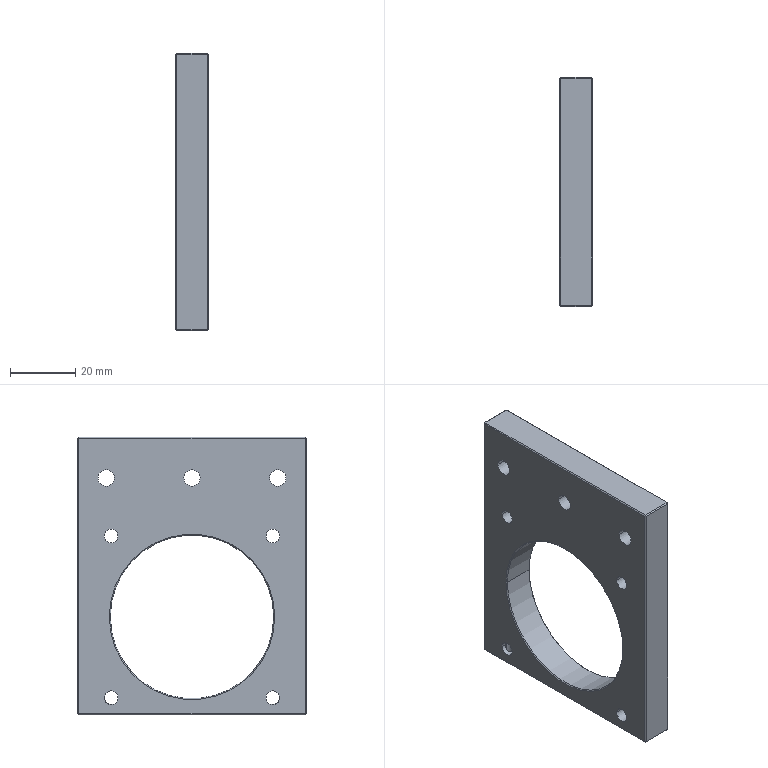Part | NX | 1 solid | 68 faces | box 10 x 70 x 85 mm | volume 38586 mm3 | cone 26 | cylinder 24 | plane 18 | commonest cylinder face diameters 2.5 x8 4.2 x8 5 x6 50 x2